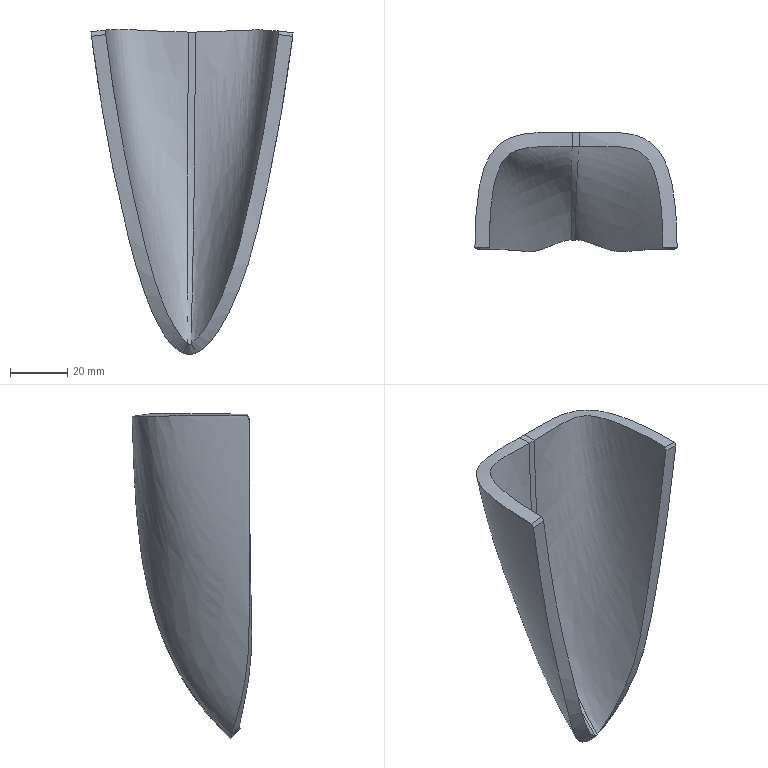Part | SolidWorks | features BaseBody 1 | 1 solid | 16 faces | box 70.874 x 41.971 x 113.991 mm | volume 48204 mm3 | spline 16